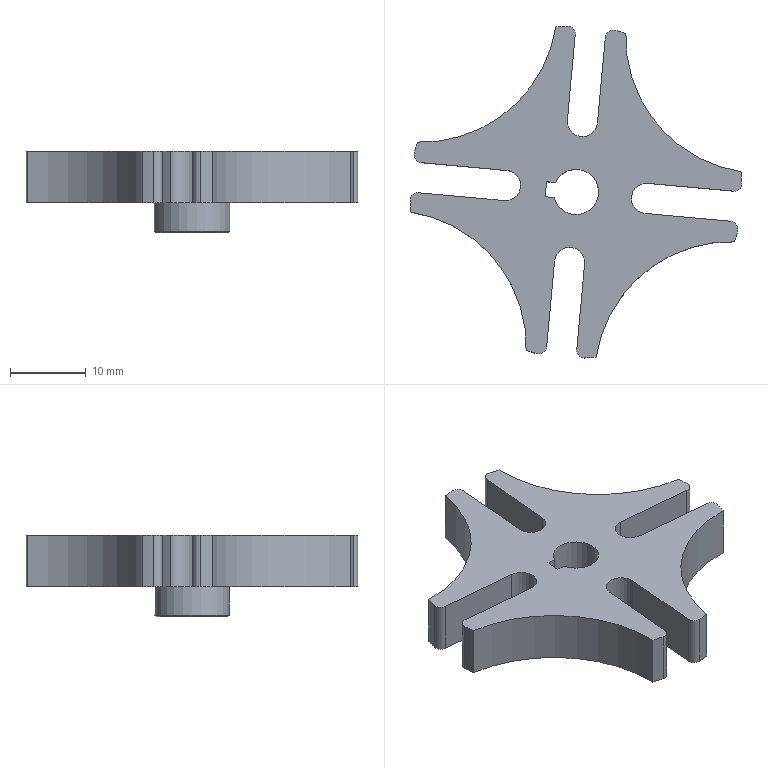Part | NX | features BREP 1, DATUM_CSYS 1 | 1 solid | 41 faces | box 43.943 x 43.943 x 10.8 mm | volume 5233 mm3 | cylinder 26 | plane 14 | cone 1 | commonest cylinder face diameters 2 x8 44 x8 4 x4 36 x4 6 x1 10 x1
STEP:
#1=CARTESIAN_POINT('',(-9.516,-1.14,4.));
#2=VERTEX_POINT('',#1);
#3=CARTESIAN_POINT('',(-9.516,-1.14,10.8));
#4=VERTEX_POINT('',#3);
#5=CARTESIAN_POINT('',(-9.516,-1.14,4.));
#6=DIRECTION('',(0.,0.,1.));
#7=VECTOR('',#6,1000.);
#8=LINE('',#5,#7);
#9=EDGE_CURVE('',#2,#4,#8,.T.);
#10=ORIENTED_EDGE('',*,*,#9,.T.);
#11=CARTESIAN_POINT('',(-9.152,2.844,10.8));
#12=VERTEX_POINT('',#11);
#13=CARTESIAN_POINT('',(-9.334,0.8521,10.8));
#14=DIRECTION('',(0.,0.,1.));
#15=DIRECTION('',(-0.09091,-0.9959,0.));
#16=AXIS2_PLACEMENT_3D('',#13,#14,#15);
#17=CIRCLE('',#16,2.);
#18=EDGE_CURVE('',#4,#12,#17,.T.);
#19=ORIENTED_EDGE('',*,*,#18,.T.);
#20=CARTESIAN_POINT('',(-9.152,2.844,4.));
#21=VERTEX_POINT('',#20);
#22=CARTESIAN_POINT('',(-9.152,2.844,4.));
#23=DIRECTION('',(0.,0.,1.));
#24=VECTOR('',#23,1000.);
#25=LINE('',#22,#24);
#26=EDGE_CURVE('',#21,#12,#25,.T.);
#27=ORIENTED_EDGE('',*,*,#26,.F.);
#28=CARTESIAN_POINT('',(-9.334,0.8521,4.));
#29=DIRECTION('',(0.,0.,1.));
#30=DIRECTION('',(-0.09091,-0.9959,0.));
#31=AXIS2_PLACEMENT_3D('',#28,#29,#30);
#32=CIRCLE('',#31,2.);
#33=EDGE_CURVE('',#2,#21,#32,.T.);
#34=ORIENTED_EDGE('',*,*,#33,.F.);
#35=EDGE_LOOP('',(#10,#19,#27,#34));
#36=FACE_BOUND('',#35,.T.);
#37=CARTESIAN_POINT('',(-9.334,0.8521,4.));
#38=DIRECTION('',(0.,0.,1.));
#39=DIRECTION('',(0.09091,0.9959,0.));
#40=AXIS2_PLACEMENT_3D('',#37,#38,#39);
#41=CYLINDRICAL_SURFACE('',#40,2.);
#42=ADVANCED_FACE('',(#36),#41,.F.);
#43=CARTESIAN_POINT('',(-21.97,-1.15,4.));
#44=VERTEX_POINT('',#43);
#45=CARTESIAN_POINT('',(-21.835,-2.689,4.));
#46=VERTEX_POINT('',#45);
#47=CARTESIAN_POINT('',(0.,0.,4.));
#48=DIRECTION('',(0.,0.,1.));
#49=DIRECTION('',(-0.9986,-0.05229,0.));
#50=AXIS2_PLACEMENT_3D('',#47,#48,#49);
#51=CIRCLE('',#50,22.);
#52=EDGE_CURVE('',#44,#46,#51,.T.);
#53=ORIENTED_EDGE('',*,*,#52,.F.);
#54=CARTESIAN_POINT('',(-20.88,-0.1022,4.));
#55=VERTEX_POINT('',#54);
#56=CARTESIAN_POINT('',(-20.971,-1.098,4.));
#57=DIRECTION('',(0.,0.,-1.));
#58=DIRECTION('',(-0.9986,-0.05229,0.));
#59=AXIS2_PLACEMENT_3D('',#56,#57,#58);
#60=CIRCLE('',#59,1.);
#61=EDGE_CURVE('',#44,#55,#60,.T.);
#62=ORIENTED_EDGE('',*,*,#61,.T.);
#63=CARTESIAN_POINT('',(-20.88,-0.1022,4.));
#64=DIRECTION('',(0.9959,-0.09091,0.));
#65=VECTOR('',#64,1000.);
#66=LINE('',#63,#65);
#67=EDGE_CURVE('',#55,#2,#66,.T.);
#68=ORIENTED_EDGE('',*,*,#67,.T.);
#69=ORIENTED_EDGE('',*,*,#33,.T.);
#70=CARTESIAN_POINT('',(-20.517,3.881,4.));
#71=VERTEX_POINT('',#70);
#72=CARTESIAN_POINT('',(-20.517,3.881,4.));
#73=DIRECTION('',(0.9959,-0.09091,0.));
#74=VECTOR('',#73,1000.);
#75=LINE('',#72,#74);
#76=EDGE_CURVE('',#71,#21,#75,.T.);
#77=ORIENTED_EDGE('',*,*,#76,.F.);
#78=CARTESIAN_POINT('',(-21.398,5.109,4.));
#79=VERTEX_POINT('',#78);
#80=CARTESIAN_POINT('',(-20.426,4.877,4.));
#81=DIRECTION('',(0.,0.,1.));
#82=DIRECTION('',(-0.9727,0.2322,0.));
#83=AXIS2_PLACEMENT_3D('',#80,#81,#82);
#84=CIRCLE('',#83,1.);
#85=EDGE_CURVE('',#79,#71,#84,.T.);
#86=ORIENTED_EDGE('',*,*,#85,.F.);
#87=CARTESIAN_POINT('',(-20.987,6.598,4.));
#88=VERTEX_POINT('',#87);
#89=CARTESIAN_POINT('',(0.,0.,4.));
#90=DIRECTION('',(0.,0.,1.));
#91=DIRECTION('',(-0.954,0.2999,0.));
#92=AXIS2_PLACEMENT_3D('',#89,#90,#91);
#93=CIRCLE('',#92,22.);
#94=EDGE_CURVE('',#88,#79,#93,.T.);
#95=ORIENTED_EDGE('',*,*,#94,.F.);
#96=CARTESIAN_POINT('',(-2.689,21.835,4.));
#97=VERTEX_POINT('',#96);
#98=CARTESIAN_POINT('',(-20.477,24.591,4.));
#99=DIRECTION('',(0.,0.,1.));
#100=DIRECTION('',(-0.02837,-0.9996,0.));
#101=AXIS2_PLACEMENT_3D('',#98,#99,#100);
#102=CIRCLE('',#101,18.);
#103=EDGE_CURVE('',#88,#97,#102,.T.);
#104=ORIENTED_EDGE('',*,*,#103,.T.);
#105=CARTESIAN_POINT('',(-1.15,21.97,4.));
#106=VERTEX_POINT('',#105);
#107=CARTESIAN_POINT('',(0.,0.,4.));
#108=DIRECTION('',(0.,0.,1.));
#109=DIRECTION('',(-0.05229,0.9986,0.));
#110=AXIS2_PLACEMENT_3D('',#107,#108,#109);
#111=CIRCLE('',#110,22.);
#112=EDGE_CURVE('',#106,#97,#111,.T.);
#113=ORIENTED_EDGE('',*,*,#112,.F.);
#114=CARTESIAN_POINT('',(-0.1022,20.88,4.));
#115=VERTEX_POINT('',#114);
#116=CARTESIAN_POINT('',(-1.098,20.971,4.));
#117=DIRECTION('',(0.,0.,-1.));
#118=DIRECTION('',(-0.05229,0.9986,0.));
#119=AXIS2_PLACEMENT_3D('',#116,#117,#118);
#120=CIRCLE('',#119,1.);
#121=EDGE_CURVE('',#106,#115,#120,.T.);
#122=ORIENTED_EDGE('',*,*,#121,.T.);
#123=CARTESIAN_POINT('',(-1.14,9.516,4.));
#124=VERTEX_POINT('',#123);
#125=CARTESIAN_POINT('',(-0.1022,20.88,4.));
#126=DIRECTION('',(-0.09091,-0.9959,0.));
#127=VECTOR('',#126,1000.);
#128=LINE('',#125,#127);
#129=EDGE_CURVE('',#115,#124,#128,.T.);
#130=ORIENTED_EDGE('',*,*,#129,.T.);
#131=CARTESIAN_POINT('',(2.844,9.152,4.));
#132=VERTEX_POINT('',#131);
#133=CARTESIAN_POINT('',(0.8521,9.334,4.));
#134=DIRECTION('',(0.,0.,1.));
#135=DIRECTION('',(-0.9959,0.09091,0.));
#136=AXIS2_PLACEMENT_3D('',#133,#134,#135);
#137=CIRCLE('',#136,2.);
#138=EDGE_CURVE('',#124,#132,#137,.T.);
#139=ORIENTED_EDGE('',*,*,#138,.T.);
#140=CARTESIAN_POINT('',(3.881,20.517,4.));
#141=VERTEX_POINT('',#140);
#142=CARTESIAN_POINT('',(3.881,20.517,4.));
#143=DIRECTION('',(-0.09091,-0.9959,0.));
#144=VECTOR('',#143,1000.);
#145=LINE('',#142,#144);
#146=EDGE_CURVE('',#141,#132,#145,.T.);
#147=ORIENTED_EDGE('',*,*,#146,.F.);
#148=CARTESIAN_POINT('',(5.109,21.398,4.));
#149=VERTEX_POINT('',#148);
#150=CARTESIAN_POINT('',(4.877,20.426,4.));
#151=DIRECTION('',(0.,0.,1.));
#152=DIRECTION('',(0.2322,0.9727,0.));
#153=AXIS2_PLACEMENT_3D('',#150,#151,#152);
#154=CIRCLE('',#153,1.);
#155=EDGE_CURVE('',#149,#141,#154,.T.);
#156=ORIENTED_EDGE('',*,*,#155,.F.);
#157=CARTESIAN_POINT('',(6.598,20.987,4.));
#158=VERTEX_POINT('',#157);
#159=CARTESIAN_POINT('',(0.,0.,4.));
#160=DIRECTION('',(0.,0.,1.));
#161=DIRECTION('',(0.2999,0.954,0.));
#162=AXIS2_PLACEMENT_3D('',#159,#160,#161);
#163=CIRCLE('',#162,22.);
#164=EDGE_CURVE('',#158,#149,#163,.T.);
#165=ORIENTED_EDGE('',*,*,#164,.F.);
#166=CARTESIAN_POINT('',(21.835,2.689,4.));
#167=VERTEX_POINT('',#166);
#168=CARTESIAN_POINT('',(24.591,20.477,4.));
#169=DIRECTION('',(0.,0.,1.));
#170=DIRECTION('',(-0.9996,0.02837,0.));
#171=AXIS2_PLACEMENT_3D('',#168,#169,#170);
#172=CIRCLE('',#171,18.);
#173=EDGE_CURVE('',#158,#167,#172,.T.);
#174=ORIENTED_EDGE('',*,*,#173,.T.);
#175=CARTESIAN_POINT('',(21.97,1.15,4.));
#176=VERTEX_POINT('',#175);
#177=CARTESIAN_POINT('',(0.,0.,4.));
#178=DIRECTION('',(0.,0.,1.));
#179=DIRECTION('',(0.9986,0.05229,0.));
#180=AXIS2_PLACEMENT_3D('',#177,#178,#179);
#181=CIRCLE('',#180,22.);
#182=EDGE_CURVE('',#176,#167,#181,.T.);
#183=ORIENTED_EDGE('',*,*,#182,.F.);
#184=CARTESIAN_POINT('',(20.88,0.1022,4.));
#185=VERTEX_POINT('',#184);
#186=CARTESIAN_POINT('',(20.971,1.098,4.));
#187=DIRECTION('',(0.,0.,-1.));
#188=DIRECTION('',(0.9986,0.05229,0.));
#189=AXIS2_PLACEMENT_3D('',#186,#187,#188);
#190=CIRCLE('',#189,1.);
#191=EDGE_CURVE('',#176,#185,#190,.T.);
#192=ORIENTED_EDGE('',*,*,#191,.T.);
#193=CARTESIAN_POINT('',(9.516,1.14,4.));
#194=VERTEX_POINT('',#193);
#195=CARTESIAN_POINT('',(20.88,0.1022,4.));
#196=DIRECTION('',(-0.9959,0.09091,0.));
#197=VECTOR('',#196,1000.);
#198=LINE('',#195,#197);
#199=EDGE_CURVE('',#185,#194,#198,.T.);
#200=ORIENTED_EDGE('',*,*,#199,.T.);
#201=CARTESIAN_POINT('',(9.152,-2.844,4.));
#202=VERTEX_POINT('',#201);
#203=CARTESIAN_POINT('',(9.334,-0.8521,4.));
#204=DIRECTION('',(0.,0.,1.));
#205=DIRECTION('',(0.09091,0.9959,0.));
#206=AXIS2_PLACEMENT_3D('',#203,#204,#205);
#207=CIRCLE('',#206,2.);
#208=EDGE_CURVE('',#194,#202,#207,.T.);
#209=ORIENTED_EDGE('',*,*,#208,.T.);
#210=CARTESIAN_POINT('',(20.517,-3.881,4.));
#211=VERTEX_POINT('',#210);
#212=CARTESIAN_POINT('',(20.517,-3.881,4.));
#213=DIRECTION('',(-0.9959,0.09091,0.));
#214=VECTOR('',#213,1000.);
#215=LINE('',#212,#214);
#216=EDGE_CURVE('',#211,#202,#215,.T.);
#217=ORIENTED_EDGE('',*,*,#216,.F.);
#218=CARTESIAN_POINT('',(21.398,-5.109,4.));
#219=VERTEX_POINT('',#218);
#220=CARTESIAN_POINT('',(20.426,-4.877,4.));
#221=DIRECTION('',(0.,0.,1.));
#222=DIRECTION('',(0.9727,-0.2322,0.));
#223=AXIS2_PLACEMENT_3D('',#220,#221,#222);
#224=CIRCLE('',#223,1.);
#225=EDGE_CURVE('',#219,#211,#224,.T.);
#226=ORIENTED_EDGE('',*,*,#225,.F.);
#227=CARTESIAN_POINT('',(20.987,-6.598,4.));
#228=VERTEX_POINT('',#227);
#229=CARTESIAN_POINT('',(0.,0.,4.));
#230=DIRECTION('',(0.,0.,1.));
#231=DIRECTION('',(0.954,-0.2999,0.));
#232=AXIS2_PLACEMENT_3D('',#229,#230,#231);
#233=CIRCLE('',#232,22.);
#234=EDGE_CURVE('',#228,#219,#233,.T.);
#235=ORIENTED_EDGE('',*,*,#234,.F.);
#236=CARTESIAN_POINT('',(2.689,-21.835,4.));
#237=VERTEX_POINT('',#236);
#238=CARTESIAN_POINT('',(20.477,-24.591,4.));
#239=DIRECTION('',(0.,0.,1.));
#240=DIRECTION('',(0.02837,0.9996,0.));
#241=AXIS2_PLACEMENT_3D('',#238,#239,#240);
#242=CIRCLE('',#241,18.);
#243=EDGE_CURVE('',#228,#237,#242,.T.);
#244=ORIENTED_EDGE('',*,*,#243,.T.);
#245=CARTESIAN_POINT('',(1.15,-21.97,4.));
#246=VERTEX_POINT('',#245);
#247=CARTESIAN_POINT('',(0.,0.,4.));
#248=DIRECTION('',(0.,0.,1.));
#249=DIRECTION('',(0.05229,-0.9986,0.));
#250=AXIS2_PLACEMENT_3D('',#247,#248,#249);
#251=CIRCLE('',#250,22.);
#252=EDGE_CURVE('',#246,#237,#251,.T.);
#253=ORIENTED_EDGE('',*,*,#252,.F.);
#254=CARTESIAN_POINT('',(0.1022,-20.88,4.));
#255=VERTEX_POINT('',#254);
#256=CARTESIAN_POINT('',(1.098,-20.971,4.));
#257=DIRECTION('',(0.,0.,-1.));
#258=DIRECTION('',(0.05229,-0.9986,0.));
#259=AXIS2_PLACEMENT_3D('',#256,#257,#258);
#260=CIRCLE('',#259,1.);
#261=EDGE_CURVE('',#246,#255,#260,.T.);
#262=ORIENTED_EDGE('',*,*,#261,.T.);
#263=CARTESIAN_POINT('',(1.14,-9.516,4.));
#264=VERTEX_POINT('',#263);
#265=CARTESIAN_POINT('',(0.1022,-20.88,4.));
#266=DIRECTION('',(0.09091,0.9959,0.));
#267=VECTOR('',#266,1000.);
#268=LINE('',#265,#267);
#269=EDGE_CURVE('',#255,#264,#268,.T.);
#270=ORIENTED_EDGE('',*,*,#269,.T.);
#271=CARTESIAN_POINT('',(-2.844,-9.152,4.));
#272=VERTEX_POINT('',#271);
#273=CARTESIAN_POINT('',(-0.8521,-9.334,4.));
#274=DIRECTION('',(0.,0.,1.));
#275=DIRECTION('',(0.9959,-0.09091,0.));
#276=AXIS2_PLACEMENT_3D('',#273,#274,#275);
#277=CIRCLE('',#276,2.);
#278=EDGE_CURVE('',#264,#272,#277,.T.);
#279=ORIENTED_EDGE('',*,*,#278,.T.);
#280=CARTESIAN_POINT('',(-3.881,-20.517,4.));
#281=VERTEX_POINT('',#280);
#282=CARTESIAN_POINT('',(-3.881,-20.517,4.));
#283=DIRECTION('',(0.09091,0.9959,0.));
#284=VECTOR('',#283,1000.);
#285=LINE('',#282,#284);
#286=EDGE_CURVE('',#281,#272,#285,.T.);
#287=ORIENTED_EDGE('',*,*,#286,.F.);
#288=CARTESIAN_POINT('',(-5.109,-21.398,4.));
#289=VERTEX_POINT('',#288);
#290=CARTESIAN_POINT('',(-4.877,-20.426,4.));
#291=DIRECTION('',(0.,0.,1.));
#292=DIRECTION('',(-0.2322,-0.9727,0.));
#293=AXIS2_PLACEMENT_3D('',#290,#291,#292);
#294=CIRCLE('',#293,1.);
#295=EDGE_CURVE('',#289,#281,#294,.T.);
#296=ORIENTED_EDGE('',*,*,#295,.F.);
#297=CARTESIAN_POINT('',(-6.598,-20.987,4.));
#298=VERTEX_POINT('',#297);
#299=CARTESIAN_POINT('',(0.,0.,4.));
#300=DIRECTION('',(0.,0.,1.));
#301=DIRECTION('',(-0.2999,-0.954,0.));
#302=AXIS2_PLACEMENT_3D('',#299,#300,#301);
#303=CIRCLE('',#302,22.);
#304=EDGE_CURVE('',#298,#289,#303,.T.);
#305=ORIENTED_EDGE('',*,*,#304,.F.);
#306=CARTESIAN_POINT('',(-24.591,-20.477,4.));
#307=DIRECTION('',(0.,0.,1.));
#308=DIRECTION('',(0.9996,-0.02837,0.));
#309=AXIS2_PLACEMENT_3D('',#306,#307,#308);
#310=CIRCLE('',#309,18.);
#311=EDGE_CURVE('',#298,#46,#310,.T.);
#312=ORIENTED_EDGE('',*,*,#311,.T.);
#313=EDGE_LOOP('',(#53,#62,#68,#69,#77,#86,#95,#104,#113,#122,#130,#139,#147,#156,#165,#174,#183,#192,#200,#209,#217,#226,#235,#244,#253,#262,#270,#279,#287,#296,#305,#312));
#314=FACE_BOUND('',#313,.T.);
#315=CARTESIAN_POINT('',(-5.,0.,4.));
#316=VERTEX_POINT('',#315);
#317=CARTESIAN_POINT('',(0.,0.,4.));
#318=DIRECTION('',(0.,0.,-1.));
#319=DIRECTION('',(-1.,0.,0.));
#320=AXIS2_PLACEMENT_3D('',#317,#318,#319);
#321=CIRCLE('',#320,5.);
#322=EDGE_CURVE('',#316,#316,#321,.T.);
#323=ORIENTED_EDGE('',*,*,#322,.F.);
#324=EDGE_LOOP('',(#323));
#325=FACE_BOUND('',#324,.T.);
#326=CARTESIAN_POINT('',(6.837,-1.44,4.));
#327=DIRECTION('',(0.,0.,1.));
#328=DIRECTION('',(0.9959,-0.09091,0.));
#329=AXIS2_PLACEMENT_3D('',#326,#327,#328);
#330=PLANE('',#329);
#331=ADVANCED_FACE('',(#314,#325),#330,.F.);
#332=CARTESIAN_POINT('',(-6.598,-20.987,10.8));
#333=VERTEX_POINT('',#332);
#334=CARTESIAN_POINT('',(-21.835,-2.689,10.8));
#335=VERTEX_POINT('',#334);
#336=CARTESIAN_POINT('',(-24.591,-20.477,10.8));
#337=DIRECTION('',(0.,0.,1.));
#338=DIRECTION('',(0.9996,-0.02837,0.));
#339=AXIS2_PLACEMENT_3D('',#336,#337,#338);
#340=CIRCLE('',#339,18.);
#341=EDGE_CURVE('',#333,#335,#340,.T.);
#342=ORIENTED_EDGE('',*,*,#341,.F.);
#343=CARTESIAN_POINT('',(-5.109,-21.398,10.8));
#344=VERTEX_POINT('',#343);
#345=CARTESIAN_POINT('',(0.,0.,10.8));
#346=DIRECTION('',(0.,0.,1.));
#347=DIRECTION('',(-0.2999,-0.954,0.));
#348=AXIS2_PLACEMENT_3D('',#345,#346,#347);
#349=CIRCLE('',#348,22.);
#350=EDGE_CURVE('',#333,#344,#349,.T.);
#351=ORIENTED_EDGE('',*,*,#350,.T.);
#352=CARTESIAN_POINT('',(-3.881,-20.517,10.8));
#353=VERTEX_POINT('',#352);
#354=CARTESIAN_POINT('',(-4.877,-20.426,10.8));
#355=DIRECTION('',(0.,0.,1.));
#356=DIRECTION('',(-0.2322,-0.9727,0.));
#357=AXIS2_PLACEMENT_3D('',#354,#355,#356);
#358=CIRCLE('',#357,1.);
#359=EDGE_CURVE('',#344,#353,#358,.T.);
#360=ORIENTED_EDGE('',*,*,#359,.T.);
#361=CARTESIAN_POINT('',(-2.844,-9.152,10.8));
#362=VERTEX_POINT('',#361);
#363=CARTESIAN_POINT('',(-3.881,-20.517,10.8));
#364=DIRECTION('',(0.09091,0.9959,0.));
#365=VECTOR('',#364,1000.);
#366=LINE('',#363,#365);
#367=EDGE_CURVE('',#353,#362,#366,.T.);
#368=ORIENTED_EDGE('',*,*,#367,.T.);
#369=CARTESIAN_POINT('',(1.14,-9.516,10.8));
#370=VERTEX_POINT('',#369);
#371=CARTESIAN_POINT('',(-0.8521,-9.334,10.8));
#372=DIRECTION('',(0.,0.,1.));
#373=DIRECTION('',(0.9959,-0.09091,0.));
#374=AXIS2_PLACEMENT_3D('',#371,#372,#373);
#375=CIRCLE('',#374,2.);
#376=EDGE_CURVE('',#370,#362,#375,.T.);
#377=ORIENTED_EDGE('',*,*,#376,.F.);
#378=CARTESIAN_POINT('',(0.1022,-20.88,10.8));
#379=VERTEX_POINT('',#378);
#380=CARTESIAN_POINT('',(0.1022,-20.88,10.8));
#381=DIRECTION('',(0.09091,0.9959,0.));
#382=VECTOR('',#381,1000.);
#383=LINE('',#380,#382);
#384=EDGE_CURVE('',#379,#370,#383,.T.);
#385=ORIENTED_EDGE('',*,*,#384,.F.);
#386=CARTESIAN_POINT('',(1.15,-21.97,10.8));
#387=VERTEX_POINT('',#386);
#388=CARTESIAN_POINT('',(1.098,-20.971,10.8));
#389=DIRECTION('',(0.,0.,-1.));
#390=DIRECTION('',(0.05229,-0.9986,0.));
#391=AXIS2_PLACEMENT_3D('',#388,#389,#390);
#392=CIRCLE('',#391,1.);
#393=EDGE_CURVE('',#387,#379,#392,.T.);
#394=ORIENTED_EDGE('',*,*,#393,.F.);
#395=CARTESIAN_POINT('',(2.689,-21.835,10.8));
#396=VERTEX_POINT('',#395);
#397=CARTESIAN_POINT('',(0.,0.,10.8));
#398=DIRECTION('',(0.,0.,1.));
#399=DIRECTION('',(0.05229,-0.9986,0.));
#400=AXIS2_PLACEMENT_3D('',#397,#398,#399);
#401=CIRCLE('',#400,22.);
#402=EDGE_CURVE('',#387,#396,#401,.T.);
#403=ORIENTED_EDGE('',*,*,#402,.T.);
#404=CARTESIAN_POINT('',(20.987,-6.598,10.8));
#405=VERTEX_POINT('',#404);
#406=CARTESIAN_POINT('',(20.477,-24.591,10.8));
#407=DIRECTION('',(0.,0.,1.));
#408=DIRECTION('',(0.02837,0.9996,0.));
#409=AXIS2_PLACEMENT_3D('',#406,#407,#408);
#410=CIRCLE('',#409,18.);
#411=EDGE_CURVE('',#405,#396,#410,.T.);
#412=ORIENTED_EDGE('',*,*,#411,.F.);
#413=CARTESIAN_POINT('',(21.398,-5.109,10.8));
#414=VERTEX_POINT('',#413);
#415=CARTESIAN_POINT('',(0.,0.,10.8));
#416=DIRECTION('',(0.,0.,1.));
#417=DIRECTION('',(0.954,-0.2999,0.));
#418=AXIS2_PLACEMENT_3D('',#415,#416,#417);
#419=CIRCLE('',#418,22.);
#420=EDGE_CURVE('',#405,#414,#419,.T.);
#421=ORIENTED_EDGE('',*,*,#420,.T.);
#422=CARTESIAN_POINT('',(20.517,-3.881,10.8));
#423=VERTEX_POINT('',#422);
#424=CARTESIAN_POINT('',(20.426,-4.877,10.8));
#425=DIRECTION('',(0.,0.,1.));
#426=DIRECTION('',(0.9727,-0.2322,0.));
#427=AXIS2_PLACEMENT_3D('',#424,#425,#426);
#428=CIRCLE('',#427,1.);
#429=EDGE_CURVE('',#414,#423,#428,.T.);
#430=ORIENTED_EDGE('',*,*,#429,.T.);
#431=CARTESIAN_POINT('',(9.152,-2.844,10.8));
#432=VERTEX_POINT('',#431);
#433=CARTESIAN_POINT('',(20.517,-3.881,10.8));
#434=DIRECTION('',(-0.9959,0.09091,0.));
#435=VECTOR('',#434,1000.);
#436=LINE('',#433,#435);
#437=EDGE_CURVE('',#423,#432,#436,.T.);
#438=ORIENTED_EDGE('',*,*,#437,.T.);
#439=CARTESIAN_POINT('',(9.516,1.14,10.8));
#440=VERTEX_POINT('',#439);
#441=CARTESIAN_POINT('',(9.334,-0.8521,10.8));
#442=DIRECTION('',(0.,0.,1.));
#443=DIRECTION('',(0.09091,0.9959,0.));
#444=AXIS2_PLACEMENT_3D('',#441,#442,#443);
#445=CIRCLE('',#444,2.);
#446=EDGE_CURVE('',#440,#432,#445,.T.);
#447=ORIENTED_EDGE('',*,*,#446,.F.);
#448=CARTESIAN_POINT('',(20.88,0.1022,10.8));
#449=VERTEX_POINT('',#448);
#450=CARTESIAN_POINT('',(20.88,0.1022,10.8));
#451=DIRECTION('',(-0.9959,0.09091,0.));
#452=VECTOR('',#451,1000.);
#453=LINE('',#450,#452);
#454=EDGE_CURVE('',#449,#440,#453,.T.);
#455=ORIENTED_EDGE('',*,*,#454,.F.);
#456=CARTESIAN_POINT('',(21.97,1.15,10.8));
#457=VERTEX_POINT('',#456);
#458=CARTESIAN_POINT('',(20.971,1.098,10.8));
#459=DIRECTION('',(0.,0.,-1.));
#460=DIRECTION('',(0.9986,0.05229,0.));
#461=AXIS2_PLACEMENT_3D('',#458,#459,#460);
#462=CIRCLE('',#461,1.);
#463=EDGE_CURVE('',#457,#449,#462,.T.);
#464=ORIENTED_EDGE('',*,*,#463,.F.);
#465=CARTESIAN_POINT('',(21.835,2.689,10.8));
#466=VERTEX_POINT('',#465);
#467=CARTESIAN_POINT('',(0.,0.,10.8));
#468=DIRECTION('',(0.,0.,1.));
#469=DIRECTION('',(0.9986,0.05229,0.));
#470=AXIS2_PLACEMENT_3D('',#467,#468,#469);
#471=CIRCLE('',#470,22.);
#472=EDGE_CURVE('',#457,#466,#471,.T.);
#473=ORIENTED_EDGE('',*,*,#472,.T.);
#474=CARTESIAN_POINT('',(6.598,20.987,10.8));
#475=VERTEX_POINT('',#474);
#476=CARTESIAN_POINT('',(24.591,20.477,10.8));
#477=DIRECTION('',(0.,0.,1.));
#478=DIRECTION('',(-0.9996,0.02837,0.));
#479=AXIS2_PLACEMENT_3D('',#476,#477,#478);
#480=CIRCLE('',#479,18.);
#481=EDGE_CURVE('',#475,#466,#480,.T.);
#482=ORIENTED_EDGE('',*,*,#481,.F.);
#483=CARTESIAN_POINT('',(5.109,21.398,10.8));
#484=VERTEX_POINT('',#483);
#485=CARTESIAN_POINT('',(0.,0.,10.8));
#486=DIRECTION('',(0.,0.,1.));
#487=DIRECTION('',(0.2999,0.954,0.));
#488=AXIS2_PLACEMENT_3D('',#485,#486,#487);
#489=CIRCLE('',#488,22.);
#490=EDGE_CURVE('',#475,#484,#489,.T.);
#491=ORIENTED_EDGE('',*,*,#490,.T.);
#492=CARTESIAN_POINT('',(3.881,20.517,10.8));
#493=VERTEX_POINT('',#492);
#494=CARTESIAN_POINT('',(4.877,20.426,10.8));
#495=DIRECTION('',(0.,0.,1.));
#496=DIRECTION('',(0.2322,0.9727,0.));
#497=AXIS2_PLACEMENT_3D('',#494,#495,#496);
#498=CIRCLE('',#497,1.);
#499=EDGE_CURVE('',#484,#493,#498,.T.);
#500=ORIENTED_EDGE('',*,*,#499,.T.);
#501=CARTESIAN_POINT('',(2.844,9.152,10.8));
#502=VERTEX_POINT('',#501);
#503=CARTESIAN_POINT('',(3.881,20.517,10.8));
#504=DIRECTION('',(-0.09091,-0.9959,0.));
#505=VECTOR('',#504,1000.);
#506=LINE('',#503,#505);
#507=EDGE_CURVE('',#493,#502,#506,.T.);
#508=ORIENTED_EDGE('',*,*,#507,.T.);
#509=CARTESIAN_POINT('',(-1.14,9.516,10.8));
#510=VERTEX_POINT('',#509);
#511=CARTESIAN_POINT('',(0.8521,9.334,10.8));
#512=DIRECTION('',(0.,0.,1.));
#513=DIRECTION('',(-0.9959,0.09091,0.));
#514=AXIS2_PLACEMENT_3D('',#511,#512,#513);
#515=CIRCLE('',#514,2.);
#516=EDGE_CURVE('',#510,#502,#515,.T.);
#517=ORIENTED_EDGE('',*,*,#516,.F.);
#518=CARTESIAN_POINT('',(-0.1022,20.88,10.8));
#519=VERTEX_POINT('',#518);
#520=CARTESIAN_POINT('',(-0.1022,20.88,10.8));
#521=DIRECTION('',(-0.09091,-0.9959,0.));
#522=VECTOR('',#521,1000.);
#523=LINE('',#520,#522);
#524=EDGE_CURVE('',#519,#510,#523,.T.);
#525=ORIENTED_EDGE('',*,*,#524,.F.);
#526=CARTESIAN_POINT('',(-1.15,21.97,10.8));
#527=VERTEX_POINT('',#526);
#528=CARTESIAN_POINT('',(-1.098,20.971,10.8));
#529=DIRECTION('',(0.,0.,-1.));
#530=DIRECTION('',(-0.05229,0.9986,0.));
#531=AXIS2_PLACEMENT_3D('',#528,#529,#530);
#532=CIRCLE('',#531,1.);
#533=EDGE_CURVE('',#527,#519,#532,.T.);
#534=ORIENTED_EDGE('',*,*,#533,.F.);
#535=CARTESIAN_POINT('',(-2.689,21.835,10.8));
#536=VERTEX_POINT('',#535);
#537=CARTESIAN_POINT('',(0.,0.,10.8));
#538=DIRECTION('',(0.,0.,1.));
#539=DIRECTION('',(-0.05229,0.9986,0.));
#540=AXIS2_PLACEMENT_3D('',#537,#538,#539);
#541=CIRCLE('',#540,22.);
#542=EDGE_CURVE('',#527,#536,#541,.T.);
#543=ORIENTED_EDGE('',*,*,#542,.T.);
#544=CARTESIAN_POINT('',(-20.987,6.598,10.8));
#545=VERTEX_POINT('',#544);
#546=CARTESIAN_POINT('',(-20.477,24.591,10.8));
#547=DIRECTION('',(0.,0.,1.));
#548=DIRECTION('',(-0.02837,-0.9996,0.));
#549=AXIS2_PLACEMENT_3D('',#546,#547,#548);
#550=CIRCLE('',#549,18.);
#551=EDGE_CURVE('',#545,#536,#550,.T.);
#552=ORIENTED_EDGE('',*,*,#551,.F.);
#553=CARTESIAN_POINT('',(-21.398,5.109,10.8));
#554=VERTEX_POINT('',#553);
#555=CARTESIAN_POINT('',(0.,0.,10.8));
#556=DIRECTION('',(0.,0.,1.));
#557=DIRECTION('',(-0.954,0.2999,0.));
#558=AXIS2_PLACEMENT_3D('',#555,#556,#557);
#559=CIRCLE('',#558,22.);
#560=EDGE_CURVE('',#545,#554,#559,.T.);
#561=ORIENTED_EDGE('',*,*,#560,.T.);
#562=CARTESIAN_POINT('',(-20.517,3.881,10.8));
#563=VERTEX_POINT('',#562);
#564=CARTESIAN_POINT('',(-20.426,4.877,10.8));
#565=DIRECTION('',(0.,0.,1.));
#566=DIRECTION('',(-0.9727,0.2322,0.));
#567=AXIS2_PLACEMENT_3D('',#564,#565,#566);
#568=CIRCLE('',#567,1.);
#569=EDGE_CURVE('',#554,#563,#568,.T.);
#570=ORIENTED_EDGE('',*,*,#569,.T.);
#571=CARTESIAN_POINT('',(-20.517,3.881,10.8));
#572=DIRECTION('',(0.9959,-0.09091,0.));
#573=VECTOR('',#572,1000.);
#574=LINE('',#571,#573);
#575=EDGE_CURVE('',#563,#12,#574,.T.);
#576=ORIENTED_EDGE('',*,*,#575,.T.);
#577=ORIENTED_EDGE('',*,*,#18,.F.);
#578=CARTESIAN_POINT('',(-20.88,-0.1022,10.8));
#579=VERTEX_POINT('',#578);
#580=CARTESIAN_POINT('',(-20.88,-0.1022,10.8));
#581=DIRECTION('',(0.9959,-0.09091,0.));
#582=VECTOR('',#581,1000.);
#583=LINE('',#580,#582);
#584=EDGE_CURVE('',#579,#4,#583,.T.);
#585=ORIENTED_EDGE('',*,*,#584,.F.);
#586=CARTESIAN_POINT('',(-21.97,-1.15,10.8));
#587=VERTEX_POINT('',#586);
#588=CARTESIAN_POINT('',(-20.971,-1.098,10.8));
#589=DIRECTION('',(0.,0.,-1.));
#590=DIRECTION('',(-0.9986,-0.05229,0.));
#591=AXIS2_PLACEMENT_3D('',#588,#589,#590);
#592=CIRCLE('',#591,1.);
#593=EDGE_CURVE('',#587,#579,#592,.T.);
#594=ORIENTED_EDGE('',*,*,#593,.F.);
#595=CARTESIAN_POINT('',(0.,0.,10.8));
#596=DIRECTION('',(0.,0.,1.));
#597=DIRECTION('',(-0.9986,-0.05229,0.));
#598=AXIS2_PLACEMENT_3D('',#595,#596,#597);
#599=CIRCLE('',#598,22.);
#600=EDGE_CURVE('',#587,#335,#599,.T.);
#601=ORIENTED_EDGE('',*,*,#600,.T.);
#602=EDGE_LOOP('',(#342,#351,#360,#368,#377,#385,#394,#403,#412,#421,#430,#438,#447,#455,#464,#473,#482,#491,#500,#508,#517,#525,#534,#543,#552,#561,#570,#576,#577,#585,#594,#601));
#603=FACE_BOUND('',#602,.T.);
#604=CARTESIAN_POINT('',(-2.726,1.253,10.8));
#605=VERTEX_POINT('',#604);
#606=CARTESIAN_POINT('',(-2.908,-0.7387,10.8));
#607=VERTEX_POINT('',#606);
#608=CARTESIAN_POINT('',(0.,0.,10.8));
#609=DIRECTION('',(0.,0.,-1.));
#610=DIRECTION('',(-0.9086,0.4177,0.));
#611=AXIS2_PLACEMENT_3D('',#608,#609,#610);
#612=CIRCLE('',#611,3.);
#613=EDGE_CURVE('',#605,#607,#612,.T.);
#614=ORIENTED_EDGE('',*,*,#613,.T.);
#615=CARTESIAN_POINT('',(-4.074,-0.6322,10.8));
#616=VERTEX_POINT('',#615);
#617=CARTESIAN_POINT('',(-4.074,-0.6322,10.8));
#618=DIRECTION('',(0.9959,-0.09091,0.));
#619=VECTOR('',#618,1000.);
#620=LINE('',#617,#619);
#621=EDGE_CURVE('',#616,#607,#620,.T.);
#622=ORIENTED_EDGE('',*,*,#621,.F.);
#623=CARTESIAN_POINT('',(-3.893,1.359,10.8));
#624=VERTEX_POINT('',#623);
#625=CARTESIAN_POINT('',(-3.893,1.359,10.8));
#626=DIRECTION('',(-0.09091,-0.9959,0.));
#627=VECTOR('',#626,1000.);
#628=LINE('',#625,#627);
#629=EDGE_CURVE('',#624,#616,#628,.T.);
#630=ORIENTED_EDGE('',*,*,#629,.F.);
#631=CARTESIAN_POINT('',(-2.726,1.253,10.8));
#632=DIRECTION('',(-0.9959,0.09091,0.));
#633=VECTOR('',#632,1000.);
#634=LINE('',#631,#633);
#635=EDGE_CURVE('',#605,#624,#634,.T.);
#636=ORIENTED_EDGE('',*,*,#635,.F.);
#637=EDGE_LOOP('',(#614,#622,#630,#636));
#638=FACE_BOUND('',#637,.T.);
#639=CARTESIAN_POINT('',(6.837,-1.44,10.8));
#640=DIRECTION('',(0.,0.,1.));
#641=DIRECTION('',(0.9959,-0.09091,0.));
#642=AXIS2_PLACEMENT_3D('',#639,#640,#641);
#643=PLANE('',#642);
#644=ADVANCED_FACE('',(#603,#638),#643,.T.);
#645=ORIENTED_EDGE('',*,*,#67,.F.);
#646=CARTESIAN_POINT('',(-20.88,-0.1022,4.));
#647=DIRECTION('',(0.,0.,1.));
#648=VECTOR('',#647,1000.);
#649=LINE('',#646,#648);
#650=EDGE_CURVE('',#55,#579,#649,.T.);
#651=ORIENTED_EDGE('',*,*,#650,.T.);
#652=ORIENTED_EDGE('',*,*,#584,.T.);
#653=ORIENTED_EDGE('',*,*,#9,.F.);
#654=EDGE_LOOP('',(#645,#651,#652,#653));
#655=FACE_BOUND('',#654,.T.);
#656=CARTESIAN_POINT('',(-18.85,-0.2875,7.785));
#657=DIRECTION('',(-0.09091,-0.9959,0.));
#658=DIRECTION('',(-0.9959,0.09091,0.));
#659=AXIS2_PLACEMENT_3D('',#656,#657,#658);
#660=PLANE('',#659);
#661=ADVANCED_FACE('',(#655),#660,.F.);
#662=ORIENTED_EDGE('',*,*,#575,.F.);
#663=CARTESIAN_POINT('',(-20.517,3.881,4.));
#664=DIRECTION('',(0.,0.,1.));
#665=VECTOR('',#664,1000.);
#666=LINE('',#663,#665);
#667=EDGE_CURVE('',#71,#563,#666,.T.);
#668=ORIENTED_EDGE('',*,*,#667,.F.);
#669=ORIENTED_EDGE('',*,*,#76,.T.);
#670=ORIENTED_EDGE('',*,*,#26,.T.);
#671=EDGE_LOOP('',(#662,#668,#669,#670));
#672=FACE_BOUND('',#671,.T.);
#673=CARTESIAN_POINT('',(-18.487,3.696,7.83));
#674=DIRECTION('',(0.09091,0.9959,0.));
#675=DIRECTION('',(0.9959,-0.09091,0.));
#676=AXIS2_PLACEMENT_3D('',#673,#674,#675);
#677=PLANE('',#676);
#678=ADVANCED_FACE('',(#672),#677,.F.);
#679=CARTESIAN_POINT('',(-6.598,-20.987,4.));
#680=DIRECTION('',(0.,0.,1.));
#681=VECTOR('',#680,1000.);
#682=LINE('',#679,#681);
#683=EDGE_CURVE('',#298,#333,#682,.T.);
#684=ORIENTED_EDGE('',*,*,#683,.T.);
#685=ORIENTED_EDGE('',*,*,#341,.T.);
#686=CARTESIAN_POINT('',(-21.835,-2.689,10.8));
#687=DIRECTION('',(0.,0.,-1.));
#688=VECTOR('',#687,1000.);
#689=LINE('',#686,#688);
#690=EDGE_CURVE('',#335,#46,#689,.T.);
#691=ORIENTED_EDGE('',*,*,#690,.T.);
#692=ORIENTED_EDGE('',*,*,#311,.F.);
#693=EDGE_LOOP('',(#684,#685,#691,#692));
#694=FACE_BOUND('',#693,.T.);
#695=CARTESIAN_POINT('',(-24.591,-20.477,4.));
#696=DIRECTION('',(0.,0.,1.));
#697=DIRECTION('',(0.9959,-0.09091,0.));
#698=AXIS2_PLACEMENT_3D('',#695,#696,#697);
#699=CYLINDRICAL_SURFACE('',#698,18.);
#700=ADVANCED_FACE('',(#694),#699,.F.);
#701=ORIENTED_EDGE('',*,*,#683,.F.);
#702=ORIENTED_EDGE('',*,*,#304,.T.);
#703=CARTESIAN_POINT('',(-5.109,-21.398,10.8));
#704=DIRECTION('',(0.,0.,-1.));
#705=VECTOR('',#704,1000.);
#706=LINE('',#703,#705);
#707=EDGE_CURVE('',#344,#289,#706,.T.);
#708=ORIENTED_EDGE('',*,*,#707,.F.);
#709=ORIENTED_EDGE('',*,*,#350,.F.);
#710=EDGE_LOOP('',(#701,#702,#708,#709));
#711=FACE_BOUND('',#710,.T.);
#712=CARTESIAN_POINT('',(0.,0.,4.));
#713=DIRECTION('',(0.,0.,1.));
#714=DIRECTION('',(0.2999,0.954,0.));
#715=AXIS2_PLACEMENT_3D('',#712,#713,#714);
#716=CYLINDRICAL_SURFACE('',#715,22.);
#717=ADVANCED_FACE('',(#711),#716,.T.);
#718=ORIENTED_EDGE('',*,*,#295,.T.);
#719=CARTESIAN_POINT('',(-3.881,-20.517,10.8));
#720=DIRECTION('',(0.,0.,-1.));
#721=VECTOR('',#720,1000.);
#722=LINE('',#719,#721);
#723=EDGE_CURVE('',#353,#281,#722,.T.);
#724=ORIENTED_EDGE('',*,*,#723,.F.);
#725=ORIENTED_EDGE('',*,*,#359,.F.);
#726=ORIENTED_EDGE('',*,*,#707,.T.);
#727=EDGE_LOOP('',(#718,#724,#725,#726));
#728=FACE_BOUND('',#727,.T.);
#729=CARTESIAN_POINT('',(-4.877,-20.426,11.48));
#730=DIRECTION('',(0.,0.,-1.));
#731=DIRECTION('',(0.2322,0.9727,0.));
#732=AXIS2_PLACEMENT_3D('',#729,#730,#731);
#733=CYLINDRICAL_SURFACE('',#732,1.);
#734=ADVANCED_FACE('',(#728),#733,.T.);
#735=ORIENTED_EDGE('',*,*,#367,.F.);
#736=ORIENTED_EDGE('',*,*,#723,.T.);
#737=ORIENTED_EDGE('',*,*,#286,.T.);
#738=CARTESIAN_POINT('',(-2.844,-9.152,4.));
#739=DIRECTION('',(0.,0.,1.));
#740=VECTOR('',#739,1000.);
#741=LINE('',#738,#740);
#742=EDGE_CURVE('',#272,#362,#741,.T.);
#743=ORIENTED_EDGE('',*,*,#742,.T.);
#744=EDGE_LOOP('',(#735,#736,#737,#743));
#745=FACE_BOUND('',#744,.T.);
#746=CARTESIAN_POINT('',(-3.696,-18.487,7.83));
#747=DIRECTION('',(-0.9959,0.09091,0.));
#748=DIRECTION('',(0.09091,0.9959,0.));
#749=AXIS2_PLACEMENT_3D('',#746,#747,#748);
#750=PLANE('',#749);
#751=ADVANCED_FACE('',(#745),#750,.F.);
#752=CARTESIAN_POINT('',(1.14,-9.516,4.));
#753=DIRECTION('',(0.,0.,1.));
#754=VECTOR('',#753,1000.);
#755=LINE('',#752,#754);
#756=EDGE_CURVE('',#264,#370,#755,.T.);
#757=ORIENTED_EDGE('',*,*,#756,.T.);
#758=ORIENTED_EDGE('',*,*,#376,.T.);
#759=ORIENTED_EDGE('',*,*,#742,.F.);
#760=ORIENTED_EDGE('',*,*,#278,.F.);
#761=EDGE_LOOP('',(#757,#758,#759,#760));
#762=FACE_BOUND('',#761,.T.);
#763=CARTESIAN_POINT('',(-0.8521,-9.334,4.));
#764=DIRECTION('',(0.,0.,1.));
#765=DIRECTION('',(-0.9959,0.09091,0.));
#766=AXIS2_PLACEMENT_3D('',#763,#764,#765);
#767=CYLINDRICAL_SURFACE('',#766,2.);
#768=ADVANCED_FACE('',(#762),#767,.F.);
#769=ORIENTED_EDGE('',*,*,#269,.F.);
#770=CARTESIAN_POINT('',(0.1022,-20.88,4.));
#771=DIRECTION('',(0.,0.,1.));
#772=VECTOR('',#771,1000.);
#773=LINE('',#770,#772);
#774=EDGE_CURVE('',#255,#379,#773,.T.);
#775=ORIENTED_EDGE('',*,*,#774,.T.);
#776=ORIENTED_EDGE('',*,*,#384,.T.);
#777=ORIENTED_EDGE('',*,*,#756,.F.);
#778=EDGE_LOOP('',(#769,#775,#776,#777));
#779=FACE_BOUND('',#778,.T.);
#780=CARTESIAN_POINT('',(0.2875,-18.85,7.785));
#781=DIRECTION('',(0.9959,-0.09091,0.));
#782=DIRECTION('',(-0.09091,-0.9959,0.));
#783=AXIS2_PLACEMENT_3D('',#780,#781,#782);
#784=PLANE('',#783);
#785=ADVANCED_FACE('',(#779),#784,.F.);
#786=ORIENTED_EDGE('',*,*,#393,.T.);
#787=ORIENTED_EDGE('',*,*,#774,.F.);
#788=ORIENTED_EDGE('',*,*,#261,.F.);
#789=CARTESIAN_POINT('',(1.15,-21.97,4.));
#790=DIRECTION('',(0.,0.,1.));
#791=VECTOR('',#790,1000.);
#792=LINE('',#789,#791);
#793=EDGE_CURVE('',#246,#387,#792,.T.);
#794=ORIENTED_EDGE('',*,*,#793,.T.);
#795=EDGE_LOOP('',(#786,#787,#788,#794));
#796=FACE_BOUND('',#795,.T.);
#797=CARTESIAN_POINT('',(1.098,-20.971,3.88));
#798=DIRECTION('',(0.,0.,1.));
#799=DIRECTION('',(-0.05229,0.9986,0.));
#800=AXIS2_PLACEMENT_3D('',#797,#798,#799);
#801=CYLINDRICAL_SURFACE('',#800,1.);
#802=ADVANCED_FACE('',(#796),#801,.T.);
#803=CARTESIAN_POINT('',(2.689,-21.835,10.8));
#804=DIRECTION('',(0.,0.,-1.));
#805=VECTOR('',#804,1000.);
#806=LINE('',#803,#805);
#807=EDGE_CURVE('',#396,#237,#806,.T.);
#808=ORIENTED_EDGE('',*,*,#807,.F.);
#809=ORIENTED_EDGE('',*,*,#402,.F.);
#810=ORIENTED_EDGE('',*,*,#793,.F.);
#811=ORIENTED_EDGE('',*,*,#252,.T.);
#812=EDGE_LOOP('',(#808,#809,#810,#811));
#813=FACE_BOUND('',#812,.T.);
#814=CARTESIAN_POINT('',(0.,0.,4.));
#815=DIRECTION('',(0.,0.,1.));
#816=DIRECTION('',(0.2999,0.954,0.));
#817=AXIS2_PLACEMENT_3D('',#814,#815,#816);
#818=CYLINDRICAL_SURFACE('',#817,22.);
#819=ADVANCED_FACE('',(#813),#818,.T.);
#820=CARTESIAN_POINT('',(20.987,-6.598,4.));
#821=DIRECTION('',(0.,0.,1.));
#822=VECTOR('',#821,1000.);
#823=LINE('',#820,#822);
#824=EDGE_CURVE('',#228,#405,#823,.T.);
#825=ORIENTED_EDGE('',*,*,#824,.T.);
#826=ORIENTED_EDGE('',*,*,#411,.T.);
#827=ORIENTED_EDGE('',*,*,#807,.T.);
#828=ORIENTED_EDGE('',*,*,#243,.F.);
#829=EDGE_LOOP('',(#825,#826,#827,#828));
#830=FACE_BOUND('',#829,.T.);
#831=CARTESIAN_POINT('',(20.477,-24.591,4.));
#832=DIRECTION('',(0.,0.,1.));
#833=DIRECTION('',(0.09091,0.9959,0.));
#834=AXIS2_PLACEMENT_3D('',#831,#832,#833);
#835=CYLINDRICAL_SURFACE('',#834,18.);
#836=ADVANCED_FACE('',(#830),#835,.F.);
#837=ORIENTED_EDGE('',*,*,#824,.F.);
#838=ORIENTED_EDGE('',*,*,#234,.T.);
#839=CARTESIAN_POINT('',(21.398,-5.109,10.8));
#840=DIRECTION('',(0.,0.,-1.));
#841=VECTOR('',#840,1000.);
#842=LINE('',#839,#841);
#843=EDGE_CURVE('',#414,#219,#842,.T.);
#844=ORIENTED_EDGE('',*,*,#843,.F.);
#845=ORIENTED_EDGE('',*,*,#420,.F.);
#846=EDGE_LOOP('',(#837,#838,#844,#845));
#847=FACE_BOUND('',#846,.T.);
#848=CARTESIAN_POINT('',(0.,0.,4.));
#849=DIRECTION('',(0.,0.,1.));
#850=DIRECTION('',(-0.954,0.2999,0.));
#851=AXIS2_PLACEMENT_3D('',#848,#849,#850);
#852=CYLINDRICAL_SURFACE('',#851,22.);
#853=ADVANCED_FACE('',(#847),#852,.T.);
#854=ORIENTED_EDGE('',*,*,#225,.T.);
#855=CARTESIAN_POINT('',(20.517,-3.881,10.8));
#856=DIRECTION('',(0.,0.,-1.));
#857=VECTOR('',#856,1000.);
#858=LINE('',#855,#857);
#859=EDGE_CURVE('',#423,#211,#858,.T.);
#860=ORIENTED_EDGE('',*,*,#859,.F.);
#861=ORIENTED_EDGE('',*,*,#429,.F.);
#862=ORIENTED_EDGE('',*,*,#843,.T.);
#863=EDGE_LOOP('',(#854,#860,#861,#862));
#864=FACE_BOUND('',#863,.T.);
#865=CARTESIAN_POINT('',(20.426,-4.877,11.48));
#866=DIRECTION('',(0.,0.,-1.));
#867=DIRECTION('',(-0.9727,0.2322,0.));
#868=AXIS2_PLACEMENT_3D('',#865,#866,#867);
#869=CYLINDRICAL_SURFACE('',#868,1.);
#870=ADVANCED_FACE('',(#864),#869,.T.);
#871=ORIENTED_EDGE('',*,*,#437,.F.);
#872=ORIENTED_EDGE('',*,*,#859,.T.);
#873=ORIENTED_EDGE('',*,*,#216,.T.);
#874=CARTESIAN_POINT('',(9.152,-2.844,4.));
#875=DIRECTION('',(0.,0.,1.));
#876=VECTOR('',#875,1000.);
#877=LINE('',#874,#876);
#878=EDGE_CURVE('',#202,#432,#877,.T.);
#879=ORIENTED_EDGE('',*,*,#878,.T.);
#880=EDGE_LOOP('',(#871,#872,#873,#879));
#881=FACE_BOUND('',#880,.T.);
#882=CARTESIAN_POINT('',(18.487,-3.696,7.83));
#883=DIRECTION('',(-0.09091,-0.9959,0.));
#884=DIRECTION('',(-0.9959,0.09091,0.));
#885=AXIS2_PLACEMENT_3D('',#882,#883,#884);
#886=PLANE('',#885);
#887=ADVANCED_FACE('',(#881),#886,.F.);
#888=CARTESIAN_POINT('',(9.516,1.14,4.));
#889=DIRECTION('',(0.,0.,1.));
#890=VECTOR('',#889,1000.);
#891=LINE('',#888,#890);
#892=EDGE_CURVE('',#194,#440,#891,.T.);
#893=ORIENTED_EDGE('',*,*,#892,.T.);
#894=ORIENTED_EDGE('',*,*,#446,.T.);
#895=ORIENTED_EDGE('',*,*,#878,.F.);
#896=ORIENTED_EDGE('',*,*,#208,.F.);
#897=EDGE_LOOP('',(#893,#894,#895,#896));
#898=FACE_BOUND('',#897,.T.);
#899=CARTESIAN_POINT('',(9.334,-0.8521,4.));
#900=DIRECTION('',(0.,0.,1.));
#901=DIRECTION('',(-0.09091,-0.9959,0.));
#902=AXIS2_PLACEMENT_3D('',#899,#900,#901);
#903=CYLINDRICAL_SURFACE('',#902,2.);
#904=ADVANCED_FACE('',(#898),#903,.F.);
#905=ORIENTED_EDGE('',*,*,#199,.F.);
#906=CARTESIAN_POINT('',(20.88,0.1022,4.));
#907=DIRECTION('',(0.,0.,1.));
#908=VECTOR('',#907,1000.);
#909=LINE('',#906,#908);
#910=EDGE_CURVE('',#185,#449,#909,.T.);
#911=ORIENTED_EDGE('',*,*,#910,.T.);
#912=ORIENTED_EDGE('',*,*,#454,.T.);
#913=ORIENTED_EDGE('',*,*,#892,.F.);
#914=EDGE_LOOP('',(#905,#911,#912,#913));
#915=FACE_BOUND('',#914,.T.);
#916=CARTESIAN_POINT('',(18.85,0.2875,7.785));
#917=DIRECTION('',(0.09091,0.9959,0.));
#918=DIRECTION('',(0.9959,-0.09091,0.));
#919=AXIS2_PLACEMENT_3D('',#916,#917,#918);
#920=PLANE('',#919);
#921=ADVANCED_FACE('',(#915),#920,.F.);
#922=ORIENTED_EDGE('',*,*,#463,.T.);
#923=ORIENTED_EDGE('',*,*,#910,.F.);
#924=ORIENTED_EDGE('',*,*,#191,.F.);
#925=CARTESIAN_POINT('',(21.97,1.15,4.));
#926=DIRECTION('',(0.,0.,1.));
#927=VECTOR('',#926,1000.);
#928=LINE('',#925,#927);
#929=EDGE_CURVE('',#176,#457,#928,.T.);
#930=ORIENTED_EDGE('',*,*,#929,.T.);
#931=EDGE_LOOP('',(#922,#923,#924,#930));
#932=FACE_BOUND('',#931,.T.);
#933=CARTESIAN_POINT('',(20.971,1.098,3.88));
#934=DIRECTION('',(0.,0.,1.));
#935=DIRECTION('',(-0.9986,-0.05229,0.));
#936=AXIS2_PLACEMENT_3D('',#933,#934,#935);
#937=CYLINDRICAL_SURFACE('',#936,1.);
#938=ADVANCED_FACE('',(#932),#937,.T.);
#939=CARTESIAN_POINT('',(21.835,2.689,10.8));
#940=DIRECTION('',(0.,0.,-1.));
#941=VECTOR('',#940,1000.);
#942=LINE('',#939,#941);
#943=EDGE_CURVE('',#466,#167,#942,.T.);
#944=ORIENTED_EDGE('',*,*,#943,.F.);
#945=ORIENTED_EDGE('',*,*,#472,.F.);
#946=ORIENTED_EDGE('',*,*,#929,.F.);
#947=ORIENTED_EDGE('',*,*,#182,.T.);
#948=EDGE_LOOP('',(#944,#945,#946,#947));
#949=FACE_BOUND('',#948,.T.);
#950=CARTESIAN_POINT('',(0.,0.,4.));
#951=DIRECTION('',(0.,0.,1.));
#952=DIRECTION('',(-0.954,0.2999,0.));
#953=AXIS2_PLACEMENT_3D('',#950,#951,#952);
#954=CYLINDRICAL_SURFACE('',#953,22.);
#955=ADVANCED_FACE('',(#949),#954,.T.);
#956=CARTESIAN_POINT('',(6.598,20.987,4.));
#957=DIRECTION('',(0.,0.,1.));
#958=VECTOR('',#957,1000.);
#959=LINE('',#956,#958);
#960=EDGE_CURVE('',#158,#475,#959,.T.);
#961=ORIENTED_EDGE('',*,*,#960,.T.);
#962=ORIENTED_EDGE('',*,*,#481,.T.);
#963=ORIENTED_EDGE('',*,*,#943,.T.);
#964=ORIENTED_EDGE('',*,*,#173,.F.);
#965=EDGE_LOOP('',(#961,#962,#963,#964));
#966=FACE_BOUND('',#965,.T.);
#967=CARTESIAN_POINT('',(24.591,20.477,4.));
#968=DIRECTION('',(0.,0.,1.));
#969=DIRECTION('',(-0.9959,0.09091,0.));
#970=AXIS2_PLACEMENT_3D('',#967,#968,#969);
#971=CYLINDRICAL_SURFACE('',#970,18.);
#972=ADVANCED_FACE('',(#966),#971,.F.);
#973=ORIENTED_EDGE('',*,*,#960,.F.);
#974=ORIENTED_EDGE('',*,*,#164,.T.);
#975=CARTESIAN_POINT('',(5.109,21.398,10.8));
#976=DIRECTION('',(0.,0.,-1.));
#977=VECTOR('',#976,1000.);
#978=LINE('',#975,#977);
#979=EDGE_CURVE('',#484,#149,#978,.T.);
#980=ORIENTED_EDGE('',*,*,#979,.F.);
#981=ORIENTED_EDGE('',*,*,#490,.F.);
#982=EDGE_LOOP('',(#973,#974,#980,#981));
#983=FACE_BOUND('',#982,.T.);
#984=CARTESIAN_POINT('',(0.,0.,4.));
#985=DIRECTION('',(0.,0.,1.));
#986=DIRECTION('',(-0.2999,-0.954,0.));
#987=AXIS2_PLACEMENT_3D('',#984,#985,#986);
#988=CYLINDRICAL_SURFACE('',#987,22.);
#989=ADVANCED_FACE('',(#983),#988,.T.);
#990=ORIENTED_EDGE('',*,*,#155,.T.);
#991=CARTESIAN_POINT('',(3.881,20.517,10.8));
#992=DIRECTION('',(0.,0.,-1.));
#993=VECTOR('',#992,1000.);
#994=LINE('',#991,#993);
#995=EDGE_CURVE('',#493,#141,#994,.T.);
#996=ORIENTED_EDGE('',*,*,#995,.F.);
#997=ORIENTED_EDGE('',*,*,#499,.F.);
#998=ORIENTED_EDGE('',*,*,#979,.T.);
#999=EDGE_LOOP('',(#990,#996,#997,#998));
#1000=FACE_BOUND('',#999,.T.);
#1001=CARTESIAN_POINT('',(4.877,20.426,11.48));
#1002=DIRECTION('',(0.,0.,-1.));
#1003=DIRECTION('',(-0.2322,-0.9727,0.));
#1004=AXIS2_PLACEMENT_3D('',#1001,#1002,#1003);
#1005=CYLINDRICAL_SURFACE('',#1004,1.);
#1006=ADVANCED_FACE('',(#1000),#1005,.T.);
#1007=ORIENTED_EDGE('',*,*,#507,.F.);
#1008=ORIENTED_EDGE('',*,*,#995,.T.);
#1009=ORIENTED_EDGE('',*,*,#146,.T.);
#1010=CARTESIAN_POINT('',(2.844,9.152,4.));
#1011=DIRECTION('',(0.,0.,1.));
#1012=VECTOR('',#1011,1000.);
#1013=LINE('',#1010,#1012);
#1014=EDGE_CURVE('',#132,#502,#1013,.T.);
#1015=ORIENTED_EDGE('',*,*,#1014,.T.);
#1016=EDGE_LOOP('',(#1007,#1008,#1009,#1015));
#1017=FACE_BOUND('',#1016,.T.);
#1018=CARTESIAN_POINT('',(3.696,18.487,7.83));
#1019=DIRECTION('',(0.9959,-0.09091,0.));
#1020=DIRECTION('',(-0.09091,-0.9959,0.));
#1021=AXIS2_PLACEMENT_3D('',#1018,#1019,#1020);
#1022=PLANE('',#1021);
#1023=ADVANCED_FACE('',(#1017),#1022,.F.);
#1024=CARTESIAN_POINT('',(-1.14,9.516,4.));
#1025=DIRECTION('',(0.,0.,1.));
#1026=VECTOR('',#1025,1000.);
#1027=LINE('',#1024,#1026);
#1028=EDGE_CURVE('',#124,#510,#1027,.T.);
#1029=ORIENTED_EDGE('',*,*,#1028,.T.);
#1030=ORIENTED_EDGE('',*,*,#516,.T.);
#1031=ORIENTED_EDGE('',*,*,#1014,.F.);
#1032=ORIENTED_EDGE('',*,*,#138,.F.);
#1033=EDGE_LOOP('',(#1029,#1030,#1031,#1032));
#1034=FACE_BOUND('',#1033,.T.);
#1035=CARTESIAN_POINT('',(0.8521,9.334,4.));
#1036=DIRECTION('',(0.,0.,1.));
#1037=DIRECTION('',(0.9959,-0.09091,0.));
#1038=AXIS2_PLACEMENT_3D('',#1035,#1036,#1037);
#1039=CYLINDRICAL_SURFACE('',#1038,2.);
#1040=ADVANCED_FACE('',(#1034),#1039,.F.);
#1041=ORIENTED_EDGE('',*,*,#129,.F.);
#1042=CARTESIAN_POINT('',(-0.1022,20.88,4.));
#1043=DIRECTION('',(0.,0.,1.));
#1044=VECTOR('',#1043,1000.);
#1045=LINE('',#1042,#1044);
#1046=EDGE_CURVE('',#115,#519,#1045,.T.);
#1047=ORIENTED_EDGE('',*,*,#1046,.T.);
#1048=ORIENTED_EDGE('',*,*,#524,.T.);
#1049=ORIENTED_EDGE('',*,*,#1028,.F.);
#1050=EDGE_LOOP('',(#1041,#1047,#1048,#1049));
#1051=FACE_BOUND('',#1050,.T.);
#1052=CARTESIAN_POINT('',(-0.2875,18.85,7.785));
#1053=DIRECTION('',(-0.9959,0.09091,0.));
#1054=DIRECTION('',(0.09091,0.9959,0.));
#1055=AXIS2_PLACEMENT_3D('',#1052,#1053,#1054);
#1056=PLANE('',#1055);
#1057=ADVANCED_FACE('',(#1051),#1056,.F.);
#1058=ORIENTED_EDGE('',*,*,#533,.T.);
#1059=ORIENTED_EDGE('',*,*,#1046,.F.);
#1060=ORIENTED_EDGE('',*,*,#121,.F.);
#1061=CARTESIAN_POINT('',(-1.15,21.97,4.));
#1062=DIRECTION('',(0.,0.,1.));
#1063=VECTOR('',#1062,1000.);
#1064=LINE('',#1061,#1063);
#1065=EDGE_CURVE('',#106,#527,#1064,.T.);
#1066=ORIENTED_EDGE('',*,*,#1065,.T.);
#1067=EDGE_LOOP('',(#1058,#1059,#1060,#1066));
#1068=FACE_BOUND('',#1067,.T.);
#1069=CARTESIAN_POINT('',(-1.098,20.971,3.88));
#1070=DIRECTION('',(0.,0.,1.));
#1071=DIRECTION('',(0.05229,-0.9986,0.));
#1072=AXIS2_PLACEMENT_3D('',#1069,#1070,#1071);
#1073=CYLINDRICAL_SURFACE('',#1072,1.);
#1074=ADVANCED_FACE('',(#1068),#1073,.T.);
#1075=CARTESIAN_POINT('',(-2.689,21.835,10.8));
#1076=DIRECTION('',(0.,0.,-1.));
#1077=VECTOR('',#1076,1000.);
#1078=LINE('',#1075,#1077);
#1079=EDGE_CURVE('',#536,#97,#1078,.T.);
#1080=ORIENTED_EDGE('',*,*,#1079,.F.);
#1081=ORIENTED_EDGE('',*,*,#542,.F.);
#1082=ORIENTED_EDGE('',*,*,#1065,.F.);
#1083=ORIENTED_EDGE('',*,*,#112,.T.);
#1084=EDGE_LOOP('',(#1080,#1081,#1082,#1083));
#1085=FACE_BOUND('',#1084,.T.);
#1086=CARTESIAN_POINT('',(0.,0.,4.));
#1087=DIRECTION('',(0.,0.,1.));
#1088=DIRECTION('',(0.,-1.,0.));
#1089=AXIS2_PLACEMENT_3D('',#1086,#1087,#1088);
#1090=CYLINDRICAL_SURFACE('',#1089,22.);
#1091=ADVANCED_FACE('',(#1085),#1090,.T.);
#1092=CARTESIAN_POINT('',(-20.987,6.598,4.));
#1093=DIRECTION('',(0.,0.,1.));
#1094=VECTOR('',#1093,1000.);
#1095=LINE('',#1092,#1094);
#1096=EDGE_CURVE('',#88,#545,#1095,.T.);
#1097=ORIENTED_EDGE('',*,*,#1096,.T.);
#1098=ORIENTED_EDGE('',*,*,#551,.T.);
#1099=ORIENTED_EDGE('',*,*,#1079,.T.);
#1100=ORIENTED_EDGE('',*,*,#103,.F.);
#1101=EDGE_LOOP('',(#1097,#1098,#1099,#1100));
#1102=FACE_BOUND('',#1101,.T.);
#1103=CARTESIAN_POINT('',(-20.477,24.591,4.));
#1104=DIRECTION('',(0.,0.,1.));
#1105=DIRECTION('',(-0.09091,-0.9959,0.));
#1106=AXIS2_PLACEMENT_3D('',#1103,#1104,#1105);
#1107=CYLINDRICAL_SURFACE('',#1106,18.);
#1108=ADVANCED_FACE('',(#1102),#1107,.F.);
#1109=ORIENTED_EDGE('',*,*,#1096,.F.);
#1110=ORIENTED_EDGE('',*,*,#94,.T.);
#1111=CARTESIAN_POINT('',(-21.398,5.109,4.));
#1112=DIRECTION('',(0.,0.,1.));
#1113=VECTOR('',#1112,1000.);
#1114=LINE('',#1111,#1113);
#1115=EDGE_CURVE('',#79,#554,#1114,.T.);
#1116=ORIENTED_EDGE('',*,*,#1115,.T.);
#1117=ORIENTED_EDGE('',*,*,#560,.F.);
#1118=EDGE_LOOP('',(#1109,#1110,#1116,#1117));
#1119=FACE_BOUND('',#1118,.T.);
#1120=CARTESIAN_POINT('',(0.,0.,4.));
#1121=DIRECTION('',(0.,0.,1.));
#1122=DIRECTION('',(0.954,-0.2999,0.));
#1123=AXIS2_PLACEMENT_3D('',#1120,#1121,#1122);
#1124=CYLINDRICAL_SURFACE('',#1123,22.);
#1125=ADVANCED_FACE('',(#1119),#1124,.T.);
#1126=ORIENTED_EDGE('',*,*,#1115,.F.);
#1127=ORIENTED_EDGE('',*,*,#85,.T.);
#1128=ORIENTED_EDGE('',*,*,#667,.T.);
#1129=ORIENTED_EDGE('',*,*,#569,.F.);
#1130=EDGE_LOOP('',(#1126,#1127,#1128,#1129));
#1131=FACE_BOUND('',#1130,.T.);
#1132=CARTESIAN_POINT('',(-20.426,4.877,3.88));
#1133=DIRECTION('',(0.,0.,1.));
#1134=DIRECTION('',(0.9727,-0.2322,0.));
#1135=AXIS2_PLACEMENT_3D('',#1132,#1133,#1134);
#1136=CYLINDRICAL_SURFACE('',#1135,1.);
#1137=ADVANCED_FACE('',(#1131),#1136,.T.);
#1138=ORIENTED_EDGE('',*,*,#593,.T.);
#1139=ORIENTED_EDGE('',*,*,#650,.F.);
#1140=ORIENTED_EDGE('',*,*,#61,.F.);
#1141=CARTESIAN_POINT('',(-21.97,-1.15,4.));
#1142=DIRECTION('',(0.,0.,1.));
#1143=VECTOR('',#1142,1000.);
#1144=LINE('',#1141,#1143);
#1145=EDGE_CURVE('',#44,#587,#1144,.T.);
#1146=ORIENTED_EDGE('',*,*,#1145,.T.);
#1147=EDGE_LOOP('',(#1138,#1139,#1140,#1146));
#1148=FACE_BOUND('',#1147,.T.);
#1149=CARTESIAN_POINT('',(-20.971,-1.098,3.88));
#1150=DIRECTION('',(0.,0.,1.));
#1151=DIRECTION('',(0.9986,0.05229,0.));
#1152=AXIS2_PLACEMENT_3D('',#1149,#1150,#1151);
#1153=CYLINDRICAL_SURFACE('',#1152,1.);
#1154=ADVANCED_FACE('',(#1148),#1153,.T.);
#1155=ORIENTED_EDGE('',*,*,#690,.F.);
#1156=ORIENTED_EDGE('',*,*,#600,.F.);
#1157=ORIENTED_EDGE('',*,*,#1145,.F.);
#1158=ORIENTED_EDGE('',*,*,#52,.T.);
#1159=EDGE_LOOP('',(#1155,#1156,#1157,#1158));
#1160=FACE_BOUND('',#1159,.T.);
#1161=CARTESIAN_POINT('',(0.,0.,4.));
#1162=DIRECTION('',(0.,0.,1.));
#1163=DIRECTION('',(1.,0.,0.));
#1164=AXIS2_PLACEMENT_3D('',#1161,#1162,#1163);
#1165=CYLINDRICAL_SURFACE('',#1164,22.);
#1166=ADVANCED_FACE('',(#1160),#1165,.T.);
#1167=ORIENTED_EDGE('',*,*,#322,.T.);
#1168=CARTESIAN_POINT('',(-5.,0.,0.2));
#1169=VERTEX_POINT('',#1168);
#1170=CARTESIAN_POINT('',(-5.,0.,4.));
#1171=DIRECTION('',(0.,0.,-1.));
#1172=VECTOR('',#1171,1000.);
#1173=LINE('',#1170,#1172);
#1174=EDGE_CURVE('',#316,#1169,#1173,.T.);
#1175=ORIENTED_EDGE('',*,*,#1174,.T.);
#1176=CARTESIAN_POINT('',(0.,0.,0.2));
#1177=DIRECTION('',(0.,0.,1.));
#1178=DIRECTION('',(-1.,0.,0.));
#1179=AXIS2_PLACEMENT_3D('',#1176,#1177,#1178);
#1180=CIRCLE('',#1179,5.);
#1181=EDGE_CURVE('',#1169,#1169,#1180,.T.);
#1182=ORIENTED_EDGE('',*,*,#1181,.T.);
#1183=ORIENTED_EDGE('',*,*,#1174,.F.);
#1184=EDGE_LOOP('',(#1167,#1175,#1182,#1183));
#1185=FACE_BOUND('',#1184,.T.);
#1186=CARTESIAN_POINT('',(0.,0.,4.));
#1187=DIRECTION('',(0.,0.,-1.));
#1188=DIRECTION('',(1.,0.,0.));
#1189=AXIS2_PLACEMENT_3D('',#1186,#1187,#1188);
#1190=CYLINDRICAL_SURFACE('',#1189,5.);
#1191=ADVANCED_FACE('',(#1185),#1190,.T.);
#1192=CARTESIAN_POINT('',(-2.908,-0.7387,0.));
#1193=VERTEX_POINT('',#1192);
#1194=CARTESIAN_POINT('',(-2.908,-0.7387,10.8));
#1195=DIRECTION('',(0.,0.,-1.));
#1196=VECTOR('',#1195,1000.);
#1197=LINE('',#1194,#1196);
#1198=EDGE_CURVE('',#607,#1193,#1197,.T.);
#1199=ORIENTED_EDGE('',*,*,#1198,.F.);
#1200=ORIENTED_EDGE('',*,*,#613,.F.);
#1201=CARTESIAN_POINT('',(-2.726,1.253,0.));
#1202=VERTEX_POINT('',#1201);
#1203=CARTESIAN_POINT('',(-2.726,1.253,0.));
#1204=DIRECTION('',(0.,0.,1.));
#1205=VECTOR('',#1204,1000.);
#1206=LINE('',#1203,#1205);
#1207=EDGE_CURVE('',#1202,#605,#1206,.T.);
#1208=ORIENTED_EDGE('',*,*,#1207,.F.);
#1209=CARTESIAN_POINT('',(0.,0.,0.));
#1210=DIRECTION('',(0.,0.,-1.));
#1211=DIRECTION('',(-0.9086,0.4177,0.));
#1212=AXIS2_PLACEMENT_3D('',#1209,#1210,#1211);
#1213=CIRCLE('',#1212,3.);
#1214=EDGE_CURVE('',#1202,#1193,#1213,.T.);
#1215=ORIENTED_EDGE('',*,*,#1214,.T.);
#1216=EDGE_LOOP('',(#1199,#1200,#1208,#1215));
#1217=FACE_BOUND('',#1216,.T.);
#1218=CARTESIAN_POINT('',(0.,0.,32.48));
#1219=DIRECTION('',(0.,0.,-1.));
#1220=DIRECTION('',(1.,0.,0.));
#1221=AXIS2_PLACEMENT_3D('',#1218,#1219,#1220);
#1222=CYLINDRICAL_SURFACE('',#1221,3.);
#1223=ADVANCED_FACE('',(#1217),#1222,.F.);
#1224=CARTESIAN_POINT('',(-4.074,-0.6322,0.));
#1225=VERTEX_POINT('',#1224);
#1226=CARTESIAN_POINT('',(-4.074,-0.6322,10.8));
#1227=DIRECTION('',(0.,0.,-1.));
#1228=VECTOR('',#1227,1000.);
#1229=LINE('',#1226,#1228);
#1230=EDGE_CURVE('',#616,#1225,#1229,.T.);
#1231=ORIENTED_EDGE('',*,*,#1230,.F.);
#1232=ORIENTED_EDGE('',*,*,#621,.T.);
#1233=ORIENTED_EDGE('',*,*,#1198,.T.);
#1234=CARTESIAN_POINT('',(-2.908,-0.7387,0.));
#1235=DIRECTION('',(-0.9959,0.09091,0.));
#1236=VECTOR('',#1235,1000.);
#1237=LINE('',#1234,#1236);
#1238=EDGE_CURVE('',#1193,#1225,#1237,.T.);
#1239=ORIENTED_EDGE('',*,*,#1238,.T.);
#1240=EDGE_LOOP('',(#1231,#1232,#1233,#1239));
#1241=FACE_BOUND('',#1240,.T.);
#1242=CARTESIAN_POINT('',(-1.866,-0.8338,-10.365));
#1243=DIRECTION('',(0.09091,0.9959,0.));
#1244=DIRECTION('',(-0.9959,0.09091,0.));
#1245=AXIS2_PLACEMENT_3D('',#1242,#1243,#1244);
#1246=PLANE('',#1245);
#1247=ADVANCED_FACE('',(#1241),#1246,.T.);
#1248=CARTESIAN_POINT('',(-3.893,1.359,0.));
#1249=VERTEX_POINT('',#1248);
#1250=CARTESIAN_POINT('',(-3.893,1.359,10.8));
#1251=DIRECTION('',(0.,0.,-1.));
#1252=VECTOR('',#1251,1000.);
#1253=LINE('',#1250,#1252);
#1254=EDGE_CURVE('',#624,#1249,#1253,.T.);
#1255=ORIENTED_EDGE('',*,*,#1254,.F.);
#1256=ORIENTED_EDGE('',*,*,#629,.T.);
#1257=ORIENTED_EDGE('',*,*,#1230,.T.);
#1258=CARTESIAN_POINT('',(-4.074,-0.6322,0.));
#1259=DIRECTION('',(0.09091,0.9959,0.));
#1260=VECTOR('',#1259,1000.);
#1261=LINE('',#1258,#1260);
#1262=EDGE_CURVE('',#1225,#1249,#1261,.T.);
#1263=ORIENTED_EDGE('',*,*,#1262,.T.);
#1264=EDGE_LOOP('',(#1255,#1256,#1257,#1263));
#1265=FACE_BOUND('',#1264,.T.);
#1266=CARTESIAN_POINT('',(-3.983,0.3636,-10.365));
#1267=DIRECTION('',(0.9959,-0.09091,0.));
#1268=DIRECTION('',(0.09091,0.9959,0.));
#1269=AXIS2_PLACEMENT_3D('',#1266,#1267,#1268);
#1270=PLANE('',#1269);
#1271=ADVANCED_FACE('',(#1265),#1270,.T.);
#1272=ORIENTED_EDGE('',*,*,#1254,.T.);
#1273=CARTESIAN_POINT('',(-3.893,1.359,0.));
#1274=DIRECTION('',(0.9959,-0.09091,0.));
#1275=VECTOR('',#1274,1000.);
#1276=LINE('',#1273,#1275);
#1277=EDGE_CURVE('',#1249,#1202,#1276,.T.);
#1278=ORIENTED_EDGE('',*,*,#1277,.T.);
#1279=ORIENTED_EDGE('',*,*,#1207,.T.);
#1280=ORIENTED_EDGE('',*,*,#635,.T.);
#1281=EDGE_LOOP('',(#1272,#1278,#1279,#1280));
#1282=FACE_BOUND('',#1281,.T.);
#1283=CARTESIAN_POINT('',(-1.908,1.178,-10.365));
#1284=DIRECTION('',(-0.09091,-0.9959,0.));
#1285=DIRECTION('',(0.9959,-0.09091,0.));
#1286=AXIS2_PLACEMENT_3D('',#1283,#1284,#1285);
#1287=PLANE('',#1286);
#1288=ADVANCED_FACE('',(#1282),#1287,.T.);
#1289=CARTESIAN_POINT('',(-4.8,0.,0.));
#1290=VERTEX_POINT('',#1289);
#1291=CARTESIAN_POINT('',(-4.8,0.,0.));
#1292=DIRECTION('',(-0.7071,0.,0.7071));
#1293=VECTOR('',#1292,1000.);
#1294=LINE('',#1291,#1293);
#1295=EDGE_CURVE('',#1290,#1169,#1294,.T.);
#1296=ORIENTED_EDGE('',*,*,#1295,.T.);
#1297=ORIENTED_EDGE('',*,*,#1181,.F.);
#1298=ORIENTED_EDGE('',*,*,#1295,.F.);
#1299=CARTESIAN_POINT('',(0.,0.,0.));
#1300=DIRECTION('',(0.,0.,1.));
#1301=DIRECTION('',(-1.,0.,0.));
#1302=AXIS2_PLACEMENT_3D('',#1299,#1300,#1301);
#1303=CIRCLE('',#1302,4.8);
#1304=EDGE_CURVE('',#1290,#1290,#1303,.T.);
#1305=ORIENTED_EDGE('',*,*,#1304,.T.);
#1306=EDGE_LOOP('',(#1296,#1297,#1298,#1305));
#1307=FACE_BOUND('',#1306,.T.);
#1308=CARTESIAN_POINT('',(0.,0.,0.));
#1309=DIRECTION('',(0.,0.,1.));
#1310=DIRECTION('',(1.,0.,0.));
#1311=AXIS2_PLACEMENT_3D('',#1308,#1309,#1310);
#1312=CONICAL_SURFACE('',#1311,4.8,0.7854);
#1313=ADVANCED_FACE('',(#1307),#1312,.T.);
#1314=ORIENTED_EDGE('',*,*,#1304,.F.);
#1315=EDGE_LOOP('',(#1314));
#1316=FACE_BOUND('',#1315,.T.);
#1317=ORIENTED_EDGE('',*,*,#1262,.F.);
#1318=ORIENTED_EDGE('',*,*,#1238,.F.);
#1319=ORIENTED_EDGE('',*,*,#1214,.F.);
#1320=ORIENTED_EDGE('',*,*,#1277,.F.);
#1321=EDGE_LOOP('',(#1317,#1318,#1319,#1320));
#1322=FACE_BOUND('',#1321,.T.);
#1323=CARTESIAN_POINT('',(0.,0.,0.));
#1324=DIRECTION('',(0.,0.,-1.));
#1325=DIRECTION('',(1.,0.,0.));
#1326=AXIS2_PLACEMENT_3D('',#1323,#1324,#1325);
#1327=PLANE('',#1326);
#1328=ADVANCED_FACE('',(#1316,#1322),#1327,.T.);
#1329=CLOSED_SHELL('',(#42,#331,#644,#661,#678,#700,#717,#734,#751,#768,#785,#802,#819,#836,#853,#870,#887,#904,#921,#938,#955,#972,#989,#1006,#1023,#1040,#1057,#1074,#1091,#1108,#1125,#1137,#1154,#1166,#1191,#1223,#1247,#1271,#1288,#1313,#1328));
#1330=MANIFOLD_SOLID_BREP('',#1329);
#1331=(LENGTH_UNIT()NAMED_UNIT(*)SI_UNIT(.MILLI.,.METRE.));
#1332=UNCERTAINTY_MEASURE_WITH_UNIT(LENGTH_MEASURE(0.00001),#1331,'','');
#1333=(NAMED_UNIT(*)PLANE_ANGLE_UNIT()SI_UNIT($,.RADIAN.));
#1334=(NAMED_UNIT(*)SI_UNIT($,.STERADIAN.)SOLID_ANGLE_UNIT());
#1335=(GEOMETRIC_REPRESENTATION_CONTEXT(3)GLOBAL_UNCERTAINTY_ASSIGNED_CONTEXT((#1332))GLOBAL_UNIT_ASSIGNED_CONTEXT((#1331,#1333,#1334))REPRESENTATION_CONTEXT('',''));
#1336=ADVANCED_BREP_SHAPE_REPRESENTATION('',(#1330),#1335);